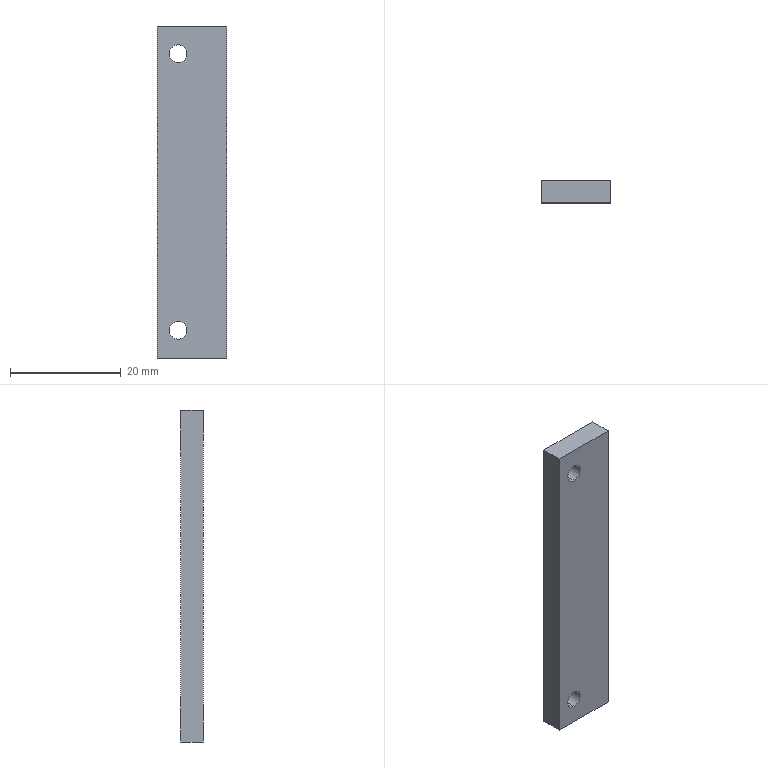Part | STEP file | PN_0027 | 1 solid | 14 faces | box 12.5 x 4 x 60 mm | volume 2901 mm3 | plane 6 | cone 4 | cylinder 4 | commonest cylinder face diameters 3.2 x4
STEP:
#1=CARTESIAN_POINT('',(0.,0.,0.));
#2=DIRECTION('',(0.,0.,1.));
#3=DIRECTION('',(1.,0.,0.));
#4=AXIS2_PLACEMENT_3D('',#1,#2,#3);
#5=CARTESIAN_POINT('',(-2.5,2.4,-23.4));
#6=VERTEX_POINT('',#5);
#7=CARTESIAN_POINT('',(-2.5,4.,-21.8));
#8=VERTEX_POINT('',#7);
#9=CARTESIAN_POINT('',(-2.5,4.,-21.8));
#10=DIRECTION('',(0.,0.7071,0.7071));
#11=VECTOR('',#10,1.);
#12=LINE('',#9,#11);
#13=CARTESIAN_POINT('',(-2.5,4.,-25.));
#14=DIRECTION('',(0.,1.,0.));
#15=DIRECTION('',(0.,0.,1.));
#16=AXIS2_PLACEMENT_3D('',#13,#14,#15);
#17=CONICAL_SURFACE('',#16,3.2,0.7854);
#18=CARTESIAN_POINT('',(6.283,0.));
#19=DIRECTION('',(0.,1.));
#20=VECTOR('',#19,1.);
#21=LINE('',#18,#20);
#22=(GEOMETRIC_REPRESENTATION_CONTEXT(2)PARAMETRIC_REPRESENTATION_CONTEXT()REPRESENTATION_CONTEXT('',''));
#23=DEFINITIONAL_REPRESENTATION('',(#21),#22);
#24=PCURVE('',#17,#23);
#25=CARTESIAN_POINT('',(-2.5,4.,-25.));
#26=DIRECTION('',(0.,1.,0.));
#27=DIRECTION('',(0.,0.,1.));
#28=AXIS2_PLACEMENT_3D('',#25,#26,#27);
#29=CONICAL_SURFACE('',#28,3.2,0.7854);
#30=CARTESIAN_POINT('',(0.,0.));
#31=DIRECTION('',(0.,1.));
#32=VECTOR('',#31,1.);
#33=LINE('',#30,#32);
#34=(GEOMETRIC_REPRESENTATION_CONTEXT(2)PARAMETRIC_REPRESENTATION_CONTEXT()REPRESENTATION_CONTEXT('',''));
#35=DEFINITIONAL_REPRESENTATION('',(#33),#34);
#36=PCURVE('',#29,#35);
#37=SURFACE_CURVE('',#12,(#24,#36),.PCURVE_S1.);
#38=EDGE_CURVE('',#6,#8,#37,.T.);
#39=ORIENTED_EDGE('',*,*,#38,.T.);
#40=CARTESIAN_POINT('',(-2.5,4.,-28.2));
#41=VERTEX_POINT('',#40);
#42=CARTESIAN_POINT('',(-2.5,4.,-25.));
#43=DIRECTION('',(0.,1.,0.));
#44=DIRECTION('',(0.,0.,1.));
#45=AXIS2_PLACEMENT_3D('',#42,#43,#44);
#46=CIRCLE('',#45,3.2);
#47=CARTESIAN_POINT('',(0.,0.));
#48=DIRECTION('',(1.,0.));
#49=VECTOR('',#48,1.);
#50=LINE('',#47,#49);
#51=(GEOMETRIC_REPRESENTATION_CONTEXT(2)PARAMETRIC_REPRESENTATION_CONTEXT()REPRESENTATION_CONTEXT('',''));
#52=DEFINITIONAL_REPRESENTATION('',(#50),#51);
#53=PCURVE('',#17,#52);
#54=CARTESIAN_POINT('',(0.,4.,0.));
#55=DIRECTION('',(0.,1.,0.));
#56=DIRECTION('',(0.,0.,1.));
#57=AXIS2_PLACEMENT_3D('',#54,#55,#56);
#58=PLANE('',#57);
#59=CARTESIAN_POINT('',(-25.,-2.5));
#60=DIRECTION('',(1.,0.));
#61=AXIS2_PLACEMENT_2D('',#59,#60);
#62=CIRCLE('',#61,3.2);
#63=(GEOMETRIC_REPRESENTATION_CONTEXT(2)PARAMETRIC_REPRESENTATION_CONTEXT()REPRESENTATION_CONTEXT('',''));
#64=DEFINITIONAL_REPRESENTATION('',(#62),#63);
#65=PCURVE('',#58,#64);
#66=SURFACE_CURVE('',#46,(#53,#65),.PCURVE_S1.);
#67=EDGE_CURVE('',#41,#8,#66,.T.);
#68=ORIENTED_EDGE('',*,*,#67,.F.);
#69=CARTESIAN_POINT('',(-2.5,2.4,-26.6));
#70=VERTEX_POINT('',#69);
#71=CARTESIAN_POINT('',(-2.5,4.,-28.2));
#72=DIRECTION('',(0.,0.7071,-0.7071));
#73=VECTOR('',#72,1.);
#74=LINE('',#71,#73);
#75=CARTESIAN_POINT('',(3.142,0.));
#76=DIRECTION('',(0.,1.));
#77=VECTOR('',#76,1.);
#78=LINE('',#75,#77);
#79=(GEOMETRIC_REPRESENTATION_CONTEXT(2)PARAMETRIC_REPRESENTATION_CONTEXT()REPRESENTATION_CONTEXT('',''));
#80=DEFINITIONAL_REPRESENTATION('',(#78),#79);
#81=PCURVE('',#17,#80);
#82=CARTESIAN_POINT('',(3.142,0.));
#83=DIRECTION('',(0.,1.));
#84=VECTOR('',#83,1.);
#85=LINE('',#82,#84);
#86=(GEOMETRIC_REPRESENTATION_CONTEXT(2)PARAMETRIC_REPRESENTATION_CONTEXT()REPRESENTATION_CONTEXT('',''));
#87=DEFINITIONAL_REPRESENTATION('',(#85),#86);
#88=PCURVE('',#29,#87);
#89=SURFACE_CURVE('',#74,(#81,#88),.PCURVE_S1.);
#90=EDGE_CURVE('',#70,#41,#89,.T.);
#91=ORIENTED_EDGE('',*,*,#90,.F.);
#92=CARTESIAN_POINT('',(-2.5,2.4,-25.));
#93=DIRECTION('',(0.,1.,0.));
#94=DIRECTION('',(0.,0.,1.));
#95=AXIS2_PLACEMENT_3D('',#92,#93,#94);
#96=CIRCLE('',#95,1.6);
#97=CARTESIAN_POINT('',(0.,-1.6));
#98=DIRECTION('',(1.,0.));
#99=VECTOR('',#98,1.);
#100=LINE('',#97,#99);
#101=(GEOMETRIC_REPRESENTATION_CONTEXT(2)PARAMETRIC_REPRESENTATION_CONTEXT()REPRESENTATION_CONTEXT('',''));
#102=DEFINITIONAL_REPRESENTATION('',(#100),#101);
#103=PCURVE('',#17,#102);
#104=CARTESIAN_POINT('',(-2.5,4.,-25.));
#105=DIRECTION('',(0.,1.,0.));
#106=DIRECTION('',(0.,0.,1.));
#107=AXIS2_PLACEMENT_3D('',#104,#105,#106);
#108=CYLINDRICAL_SURFACE('',#107,1.6);
#109=CARTESIAN_POINT('',(0.,-1.6));
#110=DIRECTION('',(1.,0.));
#111=VECTOR('',#110,1.);
#112=LINE('',#109,#111);
#113=(GEOMETRIC_REPRESENTATION_CONTEXT(2)PARAMETRIC_REPRESENTATION_CONTEXT()REPRESENTATION_CONTEXT('',''));
#114=DEFINITIONAL_REPRESENTATION('',(#112),#113);
#115=PCURVE('',#108,#114);
#116=SURFACE_CURVE('',#96,(#103,#115),.PCURVE_S1.);
#117=EDGE_CURVE('',#70,#6,#116,.T.);
#118=ORIENTED_EDGE('',*,*,#117,.T.);
#119=EDGE_LOOP('',(#39,#68,#91,#118));
#120=FACE_BOUND('',#119,.F.);
#121=ADVANCED_FACE('',(#120),#17,.F.);
#122=CARTESIAN_POINT('',(-2.5,0.,-23.4));
#123=VERTEX_POINT('',#122);
#124=CARTESIAN_POINT('',(-2.5,4.,-23.4));
#125=DIRECTION('',(0.,1.,0.));
#126=VECTOR('',#125,1.);
#127=LINE('',#124,#126);
#128=CARTESIAN_POINT('',(6.283,0.));
#129=DIRECTION('',(0.,1.));
#130=VECTOR('',#129,1.);
#131=LINE('',#128,#130);
#132=(GEOMETRIC_REPRESENTATION_CONTEXT(2)PARAMETRIC_REPRESENTATION_CONTEXT()REPRESENTATION_CONTEXT('',''));
#133=DEFINITIONAL_REPRESENTATION('',(#131),#132);
#134=PCURVE('',#108,#133);
#135=CARTESIAN_POINT('',(-2.5,4.,-25.));
#136=DIRECTION('',(0.,1.,0.));
#137=DIRECTION('',(0.,0.,1.));
#138=AXIS2_PLACEMENT_3D('',#135,#136,#137);
#139=CYLINDRICAL_SURFACE('',#138,1.6);
#140=CARTESIAN_POINT('',(0.,0.));
#141=DIRECTION('',(0.,1.));
#142=VECTOR('',#141,1.);
#143=LINE('',#140,#142);
#144=(GEOMETRIC_REPRESENTATION_CONTEXT(2)PARAMETRIC_REPRESENTATION_CONTEXT()REPRESENTATION_CONTEXT('',''));
#145=DEFINITIONAL_REPRESENTATION('',(#143),#144);
#146=PCURVE('',#139,#145);
#147=SURFACE_CURVE('',#127,(#134,#146),.PCURVE_S1.);
#148=EDGE_CURVE('',#123,#6,#147,.T.);
#149=ORIENTED_EDGE('',*,*,#148,.T.);
#150=ORIENTED_EDGE('',*,*,#117,.F.);
#151=CARTESIAN_POINT('',(-2.5,0.,-26.6));
#152=VERTEX_POINT('',#151);
#153=CARTESIAN_POINT('',(-2.5,4.,-26.6));
#154=DIRECTION('',(0.,1.,0.));
#155=VECTOR('',#154,1.);
#156=LINE('',#153,#155);
#157=CARTESIAN_POINT('',(3.142,0.));
#158=DIRECTION('',(0.,1.));
#159=VECTOR('',#158,1.);
#160=LINE('',#157,#159);
#161=(GEOMETRIC_REPRESENTATION_CONTEXT(2)PARAMETRIC_REPRESENTATION_CONTEXT()REPRESENTATION_CONTEXT('',''));
#162=DEFINITIONAL_REPRESENTATION('',(#160),#161);
#163=PCURVE('',#108,#162);
#164=CARTESIAN_POINT('',(3.142,0.));
#165=DIRECTION('',(0.,1.));
#166=VECTOR('',#165,1.);
#167=LINE('',#164,#166);
#168=(GEOMETRIC_REPRESENTATION_CONTEXT(2)PARAMETRIC_REPRESENTATION_CONTEXT()REPRESENTATION_CONTEXT('',''));
#169=DEFINITIONAL_REPRESENTATION('',(#167),#168);
#170=PCURVE('',#139,#169);
#171=SURFACE_CURVE('',#156,(#163,#170),.PCURVE_S1.);
#172=EDGE_CURVE('',#152,#70,#171,.T.);
#173=ORIENTED_EDGE('',*,*,#172,.F.);
#174=CARTESIAN_POINT('',(-2.5,0.,-25.));
#175=DIRECTION('',(0.,1.,0.));
#176=DIRECTION('',(0.,0.,1.));
#177=AXIS2_PLACEMENT_3D('',#174,#175,#176);
#178=CIRCLE('',#177,1.6);
#179=CARTESIAN_POINT('',(0.,-4.));
#180=DIRECTION('',(1.,0.));
#181=VECTOR('',#180,1.);
#182=LINE('',#179,#181);
#183=(GEOMETRIC_REPRESENTATION_CONTEXT(2)PARAMETRIC_REPRESENTATION_CONTEXT()REPRESENTATION_CONTEXT('',''));
#184=DEFINITIONAL_REPRESENTATION('',(#182),#183);
#185=PCURVE('',#108,#184);
#186=CARTESIAN_POINT('',(0.,0.,0.));
#187=DIRECTION('',(0.,1.,0.));
#188=DIRECTION('',(0.,0.,1.));
#189=AXIS2_PLACEMENT_3D('',#186,#187,#188);
#190=PLANE('',#189);
#191=CARTESIAN_POINT('',(-25.,-2.5));
#192=DIRECTION('',(1.,0.));
#193=AXIS2_PLACEMENT_2D('',#191,#192);
#194=CIRCLE('',#193,1.6);
#195=(GEOMETRIC_REPRESENTATION_CONTEXT(2)PARAMETRIC_REPRESENTATION_CONTEXT()REPRESENTATION_CONTEXT('',''));
#196=DEFINITIONAL_REPRESENTATION('',(#194),#195);
#197=PCURVE('',#190,#196);
#198=SURFACE_CURVE('',#178,(#185,#197),.PCURVE_S1.);
#199=EDGE_CURVE('',#152,#123,#198,.T.);
#200=ORIENTED_EDGE('',*,*,#199,.T.);
#201=EDGE_LOOP('',(#149,#150,#173,#200));
#202=FACE_BOUND('',#201,.F.);
#203=ADVANCED_FACE('',(#202),#108,.F.);
#204=CARTESIAN_POINT('',(-2.5,2.4,26.6));
#205=VERTEX_POINT('',#204);
#206=CARTESIAN_POINT('',(-2.5,4.,28.2));
#207=VERTEX_POINT('',#206);
#208=CARTESIAN_POINT('',(-2.5,4.,28.2));
#209=DIRECTION('',(0.,0.7071,0.7071));
#210=VECTOR('',#209,1.);
#211=LINE('',#208,#210);
#212=CARTESIAN_POINT('',(-2.5,4.,25.));
#213=DIRECTION('',(0.,1.,0.));
#214=DIRECTION('',(0.,0.,1.));
#215=AXIS2_PLACEMENT_3D('',#212,#213,#214);
#216=CONICAL_SURFACE('',#215,3.2,0.7854);
#217=CARTESIAN_POINT('',(6.283,0.));
#218=DIRECTION('',(0.,1.));
#219=VECTOR('',#218,1.);
#220=LINE('',#217,#219);
#221=(GEOMETRIC_REPRESENTATION_CONTEXT(2)PARAMETRIC_REPRESENTATION_CONTEXT()REPRESENTATION_CONTEXT('',''));
#222=DEFINITIONAL_REPRESENTATION('',(#220),#221);
#223=PCURVE('',#216,#222);
#224=CARTESIAN_POINT('',(-2.5,4.,25.));
#225=DIRECTION('',(0.,1.,0.));
#226=DIRECTION('',(0.,0.,1.));
#227=AXIS2_PLACEMENT_3D('',#224,#225,#226);
#228=CONICAL_SURFACE('',#227,3.2,0.7854);
#229=CARTESIAN_POINT('',(0.,0.));
#230=DIRECTION('',(0.,1.));
#231=VECTOR('',#230,1.);
#232=LINE('',#229,#231);
#233=(GEOMETRIC_REPRESENTATION_CONTEXT(2)PARAMETRIC_REPRESENTATION_CONTEXT()REPRESENTATION_CONTEXT('',''));
#234=DEFINITIONAL_REPRESENTATION('',(#232),#233);
#235=PCURVE('',#228,#234);
#236=SURFACE_CURVE('',#211,(#223,#235),.PCURVE_S1.);
#237=EDGE_CURVE('',#205,#207,#236,.T.);
#238=ORIENTED_EDGE('',*,*,#237,.T.);
#239=CARTESIAN_POINT('',(-2.5,4.,21.8));
#240=VERTEX_POINT('',#239);
#241=CARTESIAN_POINT('',(-2.5,4.,25.));
#242=DIRECTION('',(0.,1.,0.));
#243=DIRECTION('',(0.,0.,1.));
#244=AXIS2_PLACEMENT_3D('',#241,#242,#243);
#245=CIRCLE('',#244,3.2);
#246=CARTESIAN_POINT('',(0.,0.));
#247=DIRECTION('',(1.,0.));
#248=VECTOR('',#247,1.);
#249=LINE('',#246,#248);
#250=(GEOMETRIC_REPRESENTATION_CONTEXT(2)PARAMETRIC_REPRESENTATION_CONTEXT()REPRESENTATION_CONTEXT('',''));
#251=DEFINITIONAL_REPRESENTATION('',(#249),#250);
#252=PCURVE('',#216,#251);
#253=CARTESIAN_POINT('',(25.,-2.5));
#254=DIRECTION('',(1.,0.));
#255=AXIS2_PLACEMENT_2D('',#253,#254);
#256=CIRCLE('',#255,3.2);
#257=(GEOMETRIC_REPRESENTATION_CONTEXT(2)PARAMETRIC_REPRESENTATION_CONTEXT()REPRESENTATION_CONTEXT('',''));
#258=DEFINITIONAL_REPRESENTATION('',(#256),#257);
#259=PCURVE('',#58,#258);
#260=SURFACE_CURVE('',#245,(#252,#259),.PCURVE_S1.);
#261=EDGE_CURVE('',#240,#207,#260,.T.);
#262=ORIENTED_EDGE('',*,*,#261,.F.);
#263=CARTESIAN_POINT('',(-2.5,2.4,23.4));
#264=VERTEX_POINT('',#263);
#265=CARTESIAN_POINT('',(-2.5,4.,21.8));
#266=DIRECTION('',(0.,0.7071,-0.7071));
#267=VECTOR('',#266,1.);
#268=LINE('',#265,#267);
#269=CARTESIAN_POINT('',(3.142,0.));
#270=DIRECTION('',(0.,1.));
#271=VECTOR('',#270,1.);
#272=LINE('',#269,#271);
#273=(GEOMETRIC_REPRESENTATION_CONTEXT(2)PARAMETRIC_REPRESENTATION_CONTEXT()REPRESENTATION_CONTEXT('',''));
#274=DEFINITIONAL_REPRESENTATION('',(#272),#273);
#275=PCURVE('',#216,#274);
#276=CARTESIAN_POINT('',(3.142,0.));
#277=DIRECTION('',(0.,1.));
#278=VECTOR('',#277,1.);
#279=LINE('',#276,#278);
#280=(GEOMETRIC_REPRESENTATION_CONTEXT(2)PARAMETRIC_REPRESENTATION_CONTEXT()REPRESENTATION_CONTEXT('',''));
#281=DEFINITIONAL_REPRESENTATION('',(#279),#280);
#282=PCURVE('',#228,#281);
#283=SURFACE_CURVE('',#268,(#275,#282),.PCURVE_S1.);
#284=EDGE_CURVE('',#264,#240,#283,.T.);
#285=ORIENTED_EDGE('',*,*,#284,.F.);
#286=CARTESIAN_POINT('',(-2.5,2.4,25.));
#287=DIRECTION('',(0.,1.,0.));
#288=DIRECTION('',(0.,0.,1.));
#289=AXIS2_PLACEMENT_3D('',#286,#287,#288);
#290=CIRCLE('',#289,1.6);
#291=CARTESIAN_POINT('',(0.,-1.6));
#292=DIRECTION('',(1.,0.));
#293=VECTOR('',#292,1.);
#294=LINE('',#291,#293);
#295=(GEOMETRIC_REPRESENTATION_CONTEXT(2)PARAMETRIC_REPRESENTATION_CONTEXT()REPRESENTATION_CONTEXT('',''));
#296=DEFINITIONAL_REPRESENTATION('',(#294),#295);
#297=PCURVE('',#216,#296);
#298=CARTESIAN_POINT('',(-2.5,4.,25.));
#299=DIRECTION('',(0.,1.,0.));
#300=DIRECTION('',(0.,0.,1.));
#301=AXIS2_PLACEMENT_3D('',#298,#299,#300);
#302=CYLINDRICAL_SURFACE('',#301,1.6);
#303=CARTESIAN_POINT('',(0.,-1.6));
#304=DIRECTION('',(1.,0.));
#305=VECTOR('',#304,1.);
#306=LINE('',#303,#305);
#307=(GEOMETRIC_REPRESENTATION_CONTEXT(2)PARAMETRIC_REPRESENTATION_CONTEXT()REPRESENTATION_CONTEXT('',''));
#308=DEFINITIONAL_REPRESENTATION('',(#306),#307);
#309=PCURVE('',#302,#308);
#310=SURFACE_CURVE('',#290,(#297,#309),.PCURVE_S1.);
#311=EDGE_CURVE('',#264,#205,#310,.T.);
#312=ORIENTED_EDGE('',*,*,#311,.T.);
#313=EDGE_LOOP('',(#238,#262,#285,#312));
#314=FACE_BOUND('',#313,.F.);
#315=ADVANCED_FACE('',(#314),#216,.F.);
#316=CARTESIAN_POINT('',(-2.5,0.,26.6));
#317=VERTEX_POINT('',#316);
#318=CARTESIAN_POINT('',(-2.5,4.,26.6));
#319=DIRECTION('',(0.,1.,0.));
#320=VECTOR('',#319,1.);
#321=LINE('',#318,#320);
#322=CARTESIAN_POINT('',(6.283,0.));
#323=DIRECTION('',(0.,1.));
#324=VECTOR('',#323,1.);
#325=LINE('',#322,#324);
#326=(GEOMETRIC_REPRESENTATION_CONTEXT(2)PARAMETRIC_REPRESENTATION_CONTEXT()REPRESENTATION_CONTEXT('',''));
#327=DEFINITIONAL_REPRESENTATION('',(#325),#326);
#328=PCURVE('',#302,#327);
#329=CARTESIAN_POINT('',(-2.5,4.,25.));
#330=DIRECTION('',(0.,1.,0.));
#331=DIRECTION('',(0.,0.,1.));
#332=AXIS2_PLACEMENT_3D('',#329,#330,#331);
#333=CYLINDRICAL_SURFACE('',#332,1.6);
#334=CARTESIAN_POINT('',(0.,0.));
#335=DIRECTION('',(0.,1.));
#336=VECTOR('',#335,1.);
#337=LINE('',#334,#336);
#338=(GEOMETRIC_REPRESENTATION_CONTEXT(2)PARAMETRIC_REPRESENTATION_CONTEXT()REPRESENTATION_CONTEXT('',''));
#339=DEFINITIONAL_REPRESENTATION('',(#337),#338);
#340=PCURVE('',#333,#339);
#341=SURFACE_CURVE('',#321,(#328,#340),.PCURVE_S1.);
#342=EDGE_CURVE('',#317,#205,#341,.T.);
#343=ORIENTED_EDGE('',*,*,#342,.T.);
#344=ORIENTED_EDGE('',*,*,#311,.F.);
#345=CARTESIAN_POINT('',(-2.5,0.,23.4));
#346=VERTEX_POINT('',#345);
#347=CARTESIAN_POINT('',(-2.5,4.,23.4));
#348=DIRECTION('',(0.,1.,0.));
#349=VECTOR('',#348,1.);
#350=LINE('',#347,#349);
#351=CARTESIAN_POINT('',(3.142,0.));
#352=DIRECTION('',(0.,1.));
#353=VECTOR('',#352,1.);
#354=LINE('',#351,#353);
#355=(GEOMETRIC_REPRESENTATION_CONTEXT(2)PARAMETRIC_REPRESENTATION_CONTEXT()REPRESENTATION_CONTEXT('',''));
#356=DEFINITIONAL_REPRESENTATION('',(#354),#355);
#357=PCURVE('',#302,#356);
#358=CARTESIAN_POINT('',(3.142,0.));
#359=DIRECTION('',(0.,1.));
#360=VECTOR('',#359,1.);
#361=LINE('',#358,#360);
#362=(GEOMETRIC_REPRESENTATION_CONTEXT(2)PARAMETRIC_REPRESENTATION_CONTEXT()REPRESENTATION_CONTEXT('',''));
#363=DEFINITIONAL_REPRESENTATION('',(#361),#362);
#364=PCURVE('',#333,#363);
#365=SURFACE_CURVE('',#350,(#357,#364),.PCURVE_S1.);
#366=EDGE_CURVE('',#346,#264,#365,.T.);
#367=ORIENTED_EDGE('',*,*,#366,.F.);
#368=CARTESIAN_POINT('',(-2.5,0.,25.));
#369=DIRECTION('',(0.,1.,0.));
#370=DIRECTION('',(0.,0.,1.));
#371=AXIS2_PLACEMENT_3D('',#368,#369,#370);
#372=CIRCLE('',#371,1.6);
#373=CARTESIAN_POINT('',(0.,-4.));
#374=DIRECTION('',(1.,0.));
#375=VECTOR('',#374,1.);
#376=LINE('',#373,#375);
#377=(GEOMETRIC_REPRESENTATION_CONTEXT(2)PARAMETRIC_REPRESENTATION_CONTEXT()REPRESENTATION_CONTEXT('',''));
#378=DEFINITIONAL_REPRESENTATION('',(#376),#377);
#379=PCURVE('',#302,#378);
#380=CARTESIAN_POINT('',(25.,-2.5));
#381=DIRECTION('',(1.,0.));
#382=AXIS2_PLACEMENT_2D('',#380,#381);
#383=CIRCLE('',#382,1.6);
#384=(GEOMETRIC_REPRESENTATION_CONTEXT(2)PARAMETRIC_REPRESENTATION_CONTEXT()REPRESENTATION_CONTEXT('',''));
#385=DEFINITIONAL_REPRESENTATION('',(#383),#384);
#386=PCURVE('',#190,#385);
#387=SURFACE_CURVE('',#372,(#379,#386),.PCURVE_S1.);
#388=EDGE_CURVE('',#346,#317,#387,.T.);
#389=ORIENTED_EDGE('',*,*,#388,.T.);
#390=EDGE_LOOP('',(#343,#344,#367,#389));
#391=FACE_BOUND('',#390,.F.);
#392=ADVANCED_FACE('',(#391),#302,.F.);
#393=CARTESIAN_POINT('',(6.25,0.,30.));
#394=VERTEX_POINT('',#393);
#395=CARTESIAN_POINT('',(6.25,0.,-30.));
#396=VERTEX_POINT('',#395);
#397=CARTESIAN_POINT('',(6.25,0.,-30.));
#398=DIRECTION('',(0.,0.,-1.));
#399=VECTOR('',#398,1.);
#400=LINE('',#397,#399);
#401=CARTESIAN_POINT('',(6.25,4.,-30.));
#402=DIRECTION('',(-1.,0.,0.));
#403=DIRECTION('',(0.,0.,1.));
#404=AXIS2_PLACEMENT_3D('',#401,#402,#403);
#405=PLANE('',#404);
#406=CARTESIAN_POINT('',(0.,-4.));
#407=DIRECTION('',(-1.,0.));
#408=VECTOR('',#407,1.);
#409=LINE('',#406,#408);
#410=(GEOMETRIC_REPRESENTATION_CONTEXT(2)PARAMETRIC_REPRESENTATION_CONTEXT()REPRESENTATION_CONTEXT('',''));
#411=DEFINITIONAL_REPRESENTATION('',(#409),#410);
#412=PCURVE('',#405,#411);
#413=CARTESIAN_POINT('',(-30.,6.25));
#414=DIRECTION('',(-1.,0.));
#415=VECTOR('',#414,1.);
#416=LINE('',#413,#415);
#417=(GEOMETRIC_REPRESENTATION_CONTEXT(2)PARAMETRIC_REPRESENTATION_CONTEXT()REPRESENTATION_CONTEXT('',''));
#418=DEFINITIONAL_REPRESENTATION('',(#416),#417);
#419=PCURVE('',#190,#418);
#420=SURFACE_CURVE('',#400,(#412,#419),.PCURVE_S1.);
#421=EDGE_CURVE('',#394,#396,#420,.T.);
#422=ORIENTED_EDGE('',*,*,#421,.T.);
#423=CARTESIAN_POINT('',(6.25,4.,-30.));
#424=VERTEX_POINT('',#423);
#425=CARTESIAN_POINT('',(6.25,4.,-30.));
#426=DIRECTION('',(0.,-1.,0.));
#427=VECTOR('',#426,1.);
#428=LINE('',#425,#427);
#429=CARTESIAN_POINT('',(0.,0.));
#430=DIRECTION('',(0.,-1.));
#431=VECTOR('',#430,1.);
#432=LINE('',#429,#431);
#433=(GEOMETRIC_REPRESENTATION_CONTEXT(2)PARAMETRIC_REPRESENTATION_CONTEXT()REPRESENTATION_CONTEXT('',''));
#434=DEFINITIONAL_REPRESENTATION('',(#432),#433);
#435=PCURVE('',#405,#434);
#436=CARTESIAN_POINT('',(-6.25,4.,-30.));
#437=DIRECTION('',(0.,0.,1.));
#438=DIRECTION('',(1.,0.,0.));
#439=AXIS2_PLACEMENT_3D('',#436,#437,#438);
#440=PLANE('',#439);
#441=CARTESIAN_POINT('',(12.5,0.));
#442=DIRECTION('',(0.,-1.));
#443=VECTOR('',#442,1.);
#444=LINE('',#441,#443);
#445=(GEOMETRIC_REPRESENTATION_CONTEXT(2)PARAMETRIC_REPRESENTATION_CONTEXT()REPRESENTATION_CONTEXT('',''));
#446=DEFINITIONAL_REPRESENTATION('',(#444),#445);
#447=PCURVE('',#440,#446);
#448=SURFACE_CURVE('',#428,(#435,#447),.PCURVE_S1.);
#449=EDGE_CURVE('',#424,#396,#448,.T.);
#450=ORIENTED_EDGE('',*,*,#449,.F.);
#451=CARTESIAN_POINT('',(6.25,4.,30.));
#452=VERTEX_POINT('',#451);
#453=CARTESIAN_POINT('',(6.25,4.,-30.));
#454=DIRECTION('',(0.,0.,-1.));
#455=VECTOR('',#454,1.);
#456=LINE('',#453,#455);
#457=CARTESIAN_POINT('',(0.,0.));
#458=DIRECTION('',(-1.,0.));
#459=VECTOR('',#458,1.);
#460=LINE('',#457,#459);
#461=(GEOMETRIC_REPRESENTATION_CONTEXT(2)PARAMETRIC_REPRESENTATION_CONTEXT()REPRESENTATION_CONTEXT('',''));
#462=DEFINITIONAL_REPRESENTATION('',(#460),#461);
#463=PCURVE('',#405,#462);
#464=CARTESIAN_POINT('',(-30.,6.25));
#465=DIRECTION('',(-1.,0.));
#466=VECTOR('',#465,1.);
#467=LINE('',#464,#466);
#468=(GEOMETRIC_REPRESENTATION_CONTEXT(2)PARAMETRIC_REPRESENTATION_CONTEXT()REPRESENTATION_CONTEXT('',''));
#469=DEFINITIONAL_REPRESENTATION('',(#467),#468);
#470=PCURVE('',#58,#469);
#471=SURFACE_CURVE('',#456,(#463,#470),.PCURVE_S1.);
#472=EDGE_CURVE('',#452,#424,#471,.T.);
#473=ORIENTED_EDGE('',*,*,#472,.F.);
#474=CARTESIAN_POINT('',(6.25,4.,30.));
#475=DIRECTION('',(0.,-1.,0.));
#476=VECTOR('',#475,1.);
#477=LINE('',#474,#476);
#478=CARTESIAN_POINT('',(60.,0.));
#479=DIRECTION('',(0.,-1.));
#480=VECTOR('',#479,1.);
#481=LINE('',#478,#480);
#482=(GEOMETRIC_REPRESENTATION_CONTEXT(2)PARAMETRIC_REPRESENTATION_CONTEXT()REPRESENTATION_CONTEXT('',''));
#483=DEFINITIONAL_REPRESENTATION('',(#481),#482);
#484=PCURVE('',#405,#483);
#485=CARTESIAN_POINT('',(-6.25,4.,30.));
#486=DIRECTION('',(0.,0.,-1.));
#487=DIRECTION('',(-1.,0.,0.));
#488=AXIS2_PLACEMENT_3D('',#485,#486,#487);
#489=PLANE('',#488);
#490=CARTESIAN_POINT('',(-12.5,0.));
#491=DIRECTION('',(0.,-1.));
#492=VECTOR('',#491,1.);
#493=LINE('',#490,#492);
#494=(GEOMETRIC_REPRESENTATION_CONTEXT(2)PARAMETRIC_REPRESENTATION_CONTEXT()REPRESENTATION_CONTEXT('',''));
#495=DEFINITIONAL_REPRESENTATION('',(#493),#494);
#496=PCURVE('',#489,#495);
#497=SURFACE_CURVE('',#477,(#484,#496),.PCURVE_S1.);
#498=EDGE_CURVE('',#452,#394,#497,.T.);
#499=ORIENTED_EDGE('',*,*,#498,.T.);
#500=EDGE_LOOP('',(#422,#450,#473,#499));
#501=FACE_BOUND('',#500,.T.);
#502=ADVANCED_FACE('',(#501),#405,.F.);
#503=CARTESIAN_POINT('',(-6.25,0.,-30.));
#504=VERTEX_POINT('',#503);
#505=CARTESIAN_POINT('',(-6.25,0.,-30.));
#506=DIRECTION('',(-1.,0.,0.));
#507=VECTOR('',#506,1.);
#508=LINE('',#505,#507);
#509=CARTESIAN_POINT('',(0.,-4.));
#510=DIRECTION('',(-1.,0.));
#511=VECTOR('',#510,1.);
#512=LINE('',#509,#511);
#513=(GEOMETRIC_REPRESENTATION_CONTEXT(2)PARAMETRIC_REPRESENTATION_CONTEXT()REPRESENTATION_CONTEXT('',''));
#514=DEFINITIONAL_REPRESENTATION('',(#512),#513);
#515=PCURVE('',#440,#514);
#516=CARTESIAN_POINT('',(-30.,-6.25));
#517=DIRECTION('',(0.,-1.));
#518=VECTOR('',#517,1.);
#519=LINE('',#516,#518);
#520=(GEOMETRIC_REPRESENTATION_CONTEXT(2)PARAMETRIC_REPRESENTATION_CONTEXT()REPRESENTATION_CONTEXT('',''));
#521=DEFINITIONAL_REPRESENTATION('',(#519),#520);
#522=PCURVE('',#190,#521);
#523=SURFACE_CURVE('',#508,(#515,#522),.PCURVE_S1.);
#524=EDGE_CURVE('',#396,#504,#523,.T.);
#525=ORIENTED_EDGE('',*,*,#524,.T.);
#526=CARTESIAN_POINT('',(-6.25,4.,-30.));
#527=VERTEX_POINT('',#526);
#528=CARTESIAN_POINT('',(-6.25,4.,-30.));
#529=DIRECTION('',(0.,-1.,0.));
#530=VECTOR('',#529,1.);
#531=LINE('',#528,#530);
#532=CARTESIAN_POINT('',(0.,0.));
#533=DIRECTION('',(0.,-1.));
#534=VECTOR('',#533,1.);
#535=LINE('',#532,#534);
#536=(GEOMETRIC_REPRESENTATION_CONTEXT(2)PARAMETRIC_REPRESENTATION_CONTEXT()REPRESENTATION_CONTEXT('',''));
#537=DEFINITIONAL_REPRESENTATION('',(#535),#536);
#538=PCURVE('',#440,#537);
#539=CARTESIAN_POINT('',(-6.25,4.,-30.));
#540=DIRECTION('',(1.,0.,0.));
#541=DIRECTION('',(0.,0.,-1.));
#542=AXIS2_PLACEMENT_3D('',#539,#540,#541);
#543=PLANE('',#542);
#544=CARTESIAN_POINT('',(0.,0.));
#545=DIRECTION('',(0.,-1.));
#546=VECTOR('',#545,1.);
#547=LINE('',#544,#546);
#548=(GEOMETRIC_REPRESENTATION_CONTEXT(2)PARAMETRIC_REPRESENTATION_CONTEXT()REPRESENTATION_CONTEXT('',''));
#549=DEFINITIONAL_REPRESENTATION('',(#547),#548);
#550=PCURVE('',#543,#549);
#551=SURFACE_CURVE('',#531,(#538,#550),.PCURVE_S1.);
#552=EDGE_CURVE('',#527,#504,#551,.T.);
#553=ORIENTED_EDGE('',*,*,#552,.F.);
#554=CARTESIAN_POINT('',(-6.25,4.,-30.));
#555=DIRECTION('',(-1.,0.,0.));
#556=VECTOR('',#555,1.);
#557=LINE('',#554,#556);
#558=CARTESIAN_POINT('',(0.,0.));
#559=DIRECTION('',(-1.,0.));
#560=VECTOR('',#559,1.);
#561=LINE('',#558,#560);
#562=(GEOMETRIC_REPRESENTATION_CONTEXT(2)PARAMETRIC_REPRESENTATION_CONTEXT()REPRESENTATION_CONTEXT('',''));
#563=DEFINITIONAL_REPRESENTATION('',(#561),#562);
#564=PCURVE('',#440,#563);
#565=CARTESIAN_POINT('',(-30.,-6.25));
#566=DIRECTION('',(0.,-1.));
#567=VECTOR('',#566,1.);
#568=LINE('',#565,#567);
#569=(GEOMETRIC_REPRESENTATION_CONTEXT(2)PARAMETRIC_REPRESENTATION_CONTEXT()REPRESENTATION_CONTEXT('',''));
#570=DEFINITIONAL_REPRESENTATION('',(#568),#569);
#571=PCURVE('',#58,#570);
#572=SURFACE_CURVE('',#557,(#564,#571),.PCURVE_S1.);
#573=EDGE_CURVE('',#424,#527,#572,.T.);
#574=ORIENTED_EDGE('',*,*,#573,.F.);
#575=ORIENTED_EDGE('',*,*,#449,.T.);
#576=EDGE_LOOP('',(#525,#553,#574,#575));
#577=FACE_BOUND('',#576,.T.);
#578=ADVANCED_FACE('',(#577),#440,.F.);
#579=CARTESIAN_POINT('',(-6.25,0.,30.));
#580=VERTEX_POINT('',#579);
#581=CARTESIAN_POINT('',(-6.25,0.,-30.));
#582=DIRECTION('',(0.,0.,1.));
#583=VECTOR('',#582,1.);
#584=LINE('',#581,#583);
#585=CARTESIAN_POINT('',(0.,-4.));
#586=DIRECTION('',(-1.,0.));
#587=VECTOR('',#586,1.);
#588=LINE('',#585,#587);
#589=(GEOMETRIC_REPRESENTATION_CONTEXT(2)PARAMETRIC_REPRESENTATION_CONTEXT()REPRESENTATION_CONTEXT('',''));
#590=DEFINITIONAL_REPRESENTATION('',(#588),#589);
#591=PCURVE('',#543,#590);
#592=CARTESIAN_POINT('',(-30.,-6.25));
#593=DIRECTION('',(1.,0.));
#594=VECTOR('',#593,1.);
#595=LINE('',#592,#594);
#596=(GEOMETRIC_REPRESENTATION_CONTEXT(2)PARAMETRIC_REPRESENTATION_CONTEXT()REPRESENTATION_CONTEXT('',''));
#597=DEFINITIONAL_REPRESENTATION('',(#595),#596);
#598=PCURVE('',#190,#597);
#599=SURFACE_CURVE('',#584,(#591,#598),.PCURVE_S1.);
#600=EDGE_CURVE('',#504,#580,#599,.T.);
#601=ORIENTED_EDGE('',*,*,#600,.T.);
#602=CARTESIAN_POINT('',(-6.25,4.,30.));
#603=VERTEX_POINT('',#602);
#604=CARTESIAN_POINT('',(-6.25,4.,30.));
#605=DIRECTION('',(0.,-1.,0.));
#606=VECTOR('',#605,1.);
#607=LINE('',#604,#606);
#608=CARTESIAN_POINT('',(-60.,0.));
#609=DIRECTION('',(0.,-1.));
#610=VECTOR('',#609,1.);
#611=LINE('',#608,#610);
#612=(GEOMETRIC_REPRESENTATION_CONTEXT(2)PARAMETRIC_REPRESENTATION_CONTEXT()REPRESENTATION_CONTEXT('',''));
#613=DEFINITIONAL_REPRESENTATION('',(#611),#612);
#614=PCURVE('',#543,#613);
#615=CARTESIAN_POINT('',(0.,0.));
#616=DIRECTION('',(0.,-1.));
#617=VECTOR('',#616,1.);
#618=LINE('',#615,#617);
#619=(GEOMETRIC_REPRESENTATION_CONTEXT(2)PARAMETRIC_REPRESENTATION_CONTEXT()REPRESENTATION_CONTEXT('',''));
#620=DEFINITIONAL_REPRESENTATION('',(#618),#619);
#621=PCURVE('',#489,#620);
#622=SURFACE_CURVE('',#607,(#614,#621),.PCURVE_S1.);
#623=EDGE_CURVE('',#603,#580,#622,.T.);
#624=ORIENTED_EDGE('',*,*,#623,.F.);
#625=CARTESIAN_POINT('',(-6.25,4.,-30.));
#626=DIRECTION('',(0.,0.,1.));
#627=VECTOR('',#626,1.);
#628=LINE('',#625,#627);
#629=CARTESIAN_POINT('',(0.,0.));
#630=DIRECTION('',(-1.,0.));
#631=VECTOR('',#630,1.);
#632=LINE('',#629,#631);
#633=(GEOMETRIC_REPRESENTATION_CONTEXT(2)PARAMETRIC_REPRESENTATION_CONTEXT()REPRESENTATION_CONTEXT('',''));
#634=DEFINITIONAL_REPRESENTATION('',(#632),#633);
#635=PCURVE('',#543,#634);
#636=CARTESIAN_POINT('',(-30.,-6.25));
#637=DIRECTION('',(1.,0.));
#638=VECTOR('',#637,1.);
#639=LINE('',#636,#638);
#640=(GEOMETRIC_REPRESENTATION_CONTEXT(2)PARAMETRIC_REPRESENTATION_CONTEXT()REPRESENTATION_CONTEXT('',''));
#641=DEFINITIONAL_REPRESENTATION('',(#639),#640);
#642=PCURVE('',#58,#641);
#643=SURFACE_CURVE('',#628,(#635,#642),.PCURVE_S1.);
#644=EDGE_CURVE('',#527,#603,#643,.T.);
#645=ORIENTED_EDGE('',*,*,#644,.F.);
#646=ORIENTED_EDGE('',*,*,#552,.T.);
#647=EDGE_LOOP('',(#601,#624,#645,#646));
#648=FACE_BOUND('',#647,.T.);
#649=ADVANCED_FACE('',(#648),#543,.F.);
#650=CARTESIAN_POINT('',(-6.25,0.,30.));
#651=DIRECTION('',(1.,0.,0.));
#652=VECTOR('',#651,1.);
#653=LINE('',#650,#652);
#654=CARTESIAN_POINT('',(0.,-4.));
#655=DIRECTION('',(-1.,0.));
#656=VECTOR('',#655,1.);
#657=LINE('',#654,#656);
#658=(GEOMETRIC_REPRESENTATION_CONTEXT(2)PARAMETRIC_REPRESENTATION_CONTEXT()REPRESENTATION_CONTEXT('',''));
#659=DEFINITIONAL_REPRESENTATION('',(#657),#658);
#660=PCURVE('',#489,#659);
#661=CARTESIAN_POINT('',(30.,-6.25));
#662=DIRECTION('',(0.,1.));
#663=VECTOR('',#662,1.);
#664=LINE('',#661,#663);
#665=(GEOMETRIC_REPRESENTATION_CONTEXT(2)PARAMETRIC_REPRESENTATION_CONTEXT()REPRESENTATION_CONTEXT('',''));
#666=DEFINITIONAL_REPRESENTATION('',(#664),#665);
#667=PCURVE('',#190,#666);
#668=SURFACE_CURVE('',#653,(#660,#667),.PCURVE_S1.);
#669=EDGE_CURVE('',#580,#394,#668,.T.);
#670=ORIENTED_EDGE('',*,*,#669,.T.);
#671=ORIENTED_EDGE('',*,*,#498,.F.);
#672=CARTESIAN_POINT('',(-6.25,4.,30.));
#673=DIRECTION('',(1.,0.,0.));
#674=VECTOR('',#673,1.);
#675=LINE('',#672,#674);
#676=CARTESIAN_POINT('',(0.,0.));
#677=DIRECTION('',(-1.,0.));
#678=VECTOR('',#677,1.);
#679=LINE('',#676,#678);
#680=(GEOMETRIC_REPRESENTATION_CONTEXT(2)PARAMETRIC_REPRESENTATION_CONTEXT()REPRESENTATION_CONTEXT('',''));
#681=DEFINITIONAL_REPRESENTATION('',(#679),#680);
#682=PCURVE('',#489,#681);
#683=CARTESIAN_POINT('',(30.,-6.25));
#684=DIRECTION('',(0.,1.));
#685=VECTOR('',#684,1.);
#686=LINE('',#683,#685);
#687=(GEOMETRIC_REPRESENTATION_CONTEXT(2)PARAMETRIC_REPRESENTATION_CONTEXT()REPRESENTATION_CONTEXT('',''));
#688=DEFINITIONAL_REPRESENTATION('',(#686),#687);
#689=PCURVE('',#58,#688);
#690=SURFACE_CURVE('',#675,(#682,#689),.PCURVE_S1.);
#691=EDGE_CURVE('',#603,#452,#690,.T.);
#692=ORIENTED_EDGE('',*,*,#691,.F.);
#693=ORIENTED_EDGE('',*,*,#623,.T.);
#694=EDGE_LOOP('',(#670,#671,#692,#693));
#695=FACE_BOUND('',#694,.T.);
#696=ADVANCED_FACE('',(#695),#489,.F.);
#697=CARTESIAN_POINT('',(-2.5,4.,-25.));
#698=DIRECTION('',(0.,1.,0.));
#699=DIRECTION('',(0.,0.,1.));
#700=AXIS2_PLACEMENT_3D('',#697,#698,#699);
#701=CIRCLE('',#700,3.2);
#702=CARTESIAN_POINT('',(-25.,-2.5));
#703=DIRECTION('',(1.,0.));
#704=AXIS2_PLACEMENT_2D('',#702,#703);
#705=CIRCLE('',#704,3.2);
#706=(GEOMETRIC_REPRESENTATION_CONTEXT(2)PARAMETRIC_REPRESENTATION_CONTEXT()REPRESENTATION_CONTEXT('',''));
#707=DEFINITIONAL_REPRESENTATION('',(#705),#706);
#708=PCURVE('',#58,#707);
#709=CARTESIAN_POINT('',(0.,0.));
#710=DIRECTION('',(1.,0.));
#711=VECTOR('',#710,1.);
#712=LINE('',#709,#711);
#713=(GEOMETRIC_REPRESENTATION_CONTEXT(2)PARAMETRIC_REPRESENTATION_CONTEXT()REPRESENTATION_CONTEXT('',''));
#714=DEFINITIONAL_REPRESENTATION('',(#712),#713);
#715=PCURVE('',#29,#714);
#716=SURFACE_CURVE('',#701,(#708,#715),.PCURVE_S1.);
#717=EDGE_CURVE('',#8,#41,#716,.T.);
#718=ORIENTED_EDGE('',*,*,#717,.F.);
#719=ORIENTED_EDGE('',*,*,#67,.F.);
#720=EDGE_LOOP('',(#718,#719));
#721=FACE_BOUND('',#720,.T.);
#722=CARTESIAN_POINT('',(-2.5,4.,25.));
#723=DIRECTION('',(0.,1.,0.));
#724=DIRECTION('',(0.,0.,1.));
#725=AXIS2_PLACEMENT_3D('',#722,#723,#724);
#726=CIRCLE('',#725,3.2);
#727=CARTESIAN_POINT('',(25.,-2.5));
#728=DIRECTION('',(1.,0.));
#729=AXIS2_PLACEMENT_2D('',#727,#728);
#730=CIRCLE('',#729,3.2);
#731=(GEOMETRIC_REPRESENTATION_CONTEXT(2)PARAMETRIC_REPRESENTATION_CONTEXT()REPRESENTATION_CONTEXT('',''));
#732=DEFINITIONAL_REPRESENTATION('',(#730),#731);
#733=PCURVE('',#58,#732);
#734=CARTESIAN_POINT('',(0.,0.));
#735=DIRECTION('',(1.,0.));
#736=VECTOR('',#735,1.);
#737=LINE('',#734,#736);
#738=(GEOMETRIC_REPRESENTATION_CONTEXT(2)PARAMETRIC_REPRESENTATION_CONTEXT()REPRESENTATION_CONTEXT('',''));
#739=DEFINITIONAL_REPRESENTATION('',(#737),#738);
#740=PCURVE('',#228,#739);
#741=SURFACE_CURVE('',#726,(#733,#740),.PCURVE_S1.);
#742=EDGE_CURVE('',#207,#240,#741,.T.);
#743=ORIENTED_EDGE('',*,*,#742,.F.);
#744=ORIENTED_EDGE('',*,*,#261,.F.);
#745=EDGE_LOOP('',(#743,#744));
#746=FACE_BOUND('',#745,.T.);
#747=ORIENTED_EDGE('',*,*,#472,.T.);
#748=ORIENTED_EDGE('',*,*,#573,.T.);
#749=ORIENTED_EDGE('',*,*,#644,.T.);
#750=ORIENTED_EDGE('',*,*,#691,.T.);
#751=EDGE_LOOP('',(#747,#748,#749,#750));
#752=FACE_BOUND('',#751,.T.);
#753=ADVANCED_FACE('',(#721,#746,#752),#58,.T.);
#754=CARTESIAN_POINT('',(-2.5,0.,-25.));
#755=DIRECTION('',(0.,1.,0.));
#756=DIRECTION('',(0.,0.,1.));
#757=AXIS2_PLACEMENT_3D('',#754,#755,#756);
#758=CIRCLE('',#757,1.6);
#759=CARTESIAN_POINT('',(-25.,-2.5));
#760=DIRECTION('',(1.,0.));
#761=AXIS2_PLACEMENT_2D('',#759,#760);
#762=CIRCLE('',#761,1.6);
#763=(GEOMETRIC_REPRESENTATION_CONTEXT(2)PARAMETRIC_REPRESENTATION_CONTEXT()REPRESENTATION_CONTEXT('',''));
#764=DEFINITIONAL_REPRESENTATION('',(#762),#763);
#765=PCURVE('',#190,#764);
#766=CARTESIAN_POINT('',(0.,-4.));
#767=DIRECTION('',(1.,0.));
#768=VECTOR('',#767,1.);
#769=LINE('',#766,#768);
#770=(GEOMETRIC_REPRESENTATION_CONTEXT(2)PARAMETRIC_REPRESENTATION_CONTEXT()REPRESENTATION_CONTEXT('',''));
#771=DEFINITIONAL_REPRESENTATION('',(#769),#770);
#772=PCURVE('',#139,#771);
#773=SURFACE_CURVE('',#758,(#765,#772),.PCURVE_S1.);
#774=EDGE_CURVE('',#123,#152,#773,.T.);
#775=ORIENTED_EDGE('',*,*,#774,.T.);
#776=ORIENTED_EDGE('',*,*,#199,.T.);
#777=EDGE_LOOP('',(#775,#776));
#778=FACE_BOUND('',#777,.T.);
#779=CARTESIAN_POINT('',(-2.5,0.,25.));
#780=DIRECTION('',(0.,1.,0.));
#781=DIRECTION('',(0.,0.,1.));
#782=AXIS2_PLACEMENT_3D('',#779,#780,#781);
#783=CIRCLE('',#782,1.6);
#784=CARTESIAN_POINT('',(25.,-2.5));
#785=DIRECTION('',(1.,0.));
#786=AXIS2_PLACEMENT_2D('',#784,#785);
#787=CIRCLE('',#786,1.6);
#788=(GEOMETRIC_REPRESENTATION_CONTEXT(2)PARAMETRIC_REPRESENTATION_CONTEXT()REPRESENTATION_CONTEXT('',''));
#789=DEFINITIONAL_REPRESENTATION('',(#787),#788);
#790=PCURVE('',#190,#789);
#791=CARTESIAN_POINT('',(0.,-4.));
#792=DIRECTION('',(1.,0.));
#793=VECTOR('',#792,1.);
#794=LINE('',#791,#793);
#795=(GEOMETRIC_REPRESENTATION_CONTEXT(2)PARAMETRIC_REPRESENTATION_CONTEXT()REPRESENTATION_CONTEXT('',''));
#796=DEFINITIONAL_REPRESENTATION('',(#794),#795);
#797=PCURVE('',#333,#796);
#798=SURFACE_CURVE('',#783,(#790,#797),.PCURVE_S1.);
#799=EDGE_CURVE('',#317,#346,#798,.T.);
#800=ORIENTED_EDGE('',*,*,#799,.T.);
#801=ORIENTED_EDGE('',*,*,#388,.T.);
#802=EDGE_LOOP('',(#800,#801));
#803=FACE_BOUND('',#802,.T.);
#804=ORIENTED_EDGE('',*,*,#421,.F.);
#805=ORIENTED_EDGE('',*,*,#669,.F.);
#806=ORIENTED_EDGE('',*,*,#600,.F.);
#807=ORIENTED_EDGE('',*,*,#524,.F.);
#808=EDGE_LOOP('',(#804,#805,#806,#807));
#809=FACE_BOUND('',#808,.T.);
#810=ADVANCED_FACE('',(#778,#803,#809),#190,.F.);
#811=CARTESIAN_POINT('',(-2.5,2.4,25.));
#812=DIRECTION('',(0.,1.,0.));
#813=DIRECTION('',(0.,0.,1.));
#814=AXIS2_PLACEMENT_3D('',#811,#812,#813);
#815=CIRCLE('',#814,1.6);
#816=CARTESIAN_POINT('',(0.,-1.6));
#817=DIRECTION('',(1.,0.));
#818=VECTOR('',#817,1.);
#819=LINE('',#816,#818);
#820=(GEOMETRIC_REPRESENTATION_CONTEXT(2)PARAMETRIC_REPRESENTATION_CONTEXT()REPRESENTATION_CONTEXT('',''));
#821=DEFINITIONAL_REPRESENTATION('',(#819),#820);
#822=PCURVE('',#333,#821);
#823=CARTESIAN_POINT('',(0.,-1.6));
#824=DIRECTION('',(1.,0.));
#825=VECTOR('',#824,1.);
#826=LINE('',#823,#825);
#827=(GEOMETRIC_REPRESENTATION_CONTEXT(2)PARAMETRIC_REPRESENTATION_CONTEXT()REPRESENTATION_CONTEXT('',''));
#828=DEFINITIONAL_REPRESENTATION('',(#826),#827);
#829=PCURVE('',#228,#828);
#830=SURFACE_CURVE('',#815,(#822,#829),.PCURVE_S1.);
#831=EDGE_CURVE('',#205,#264,#830,.T.);
#832=ORIENTED_EDGE('',*,*,#831,.F.);
#833=ORIENTED_EDGE('',*,*,#342,.F.);
#834=ORIENTED_EDGE('',*,*,#799,.T.);
#835=ORIENTED_EDGE('',*,*,#366,.T.);
#836=EDGE_LOOP('',(#832,#833,#834,#835));
#837=FACE_BOUND('',#836,.F.);
#838=ADVANCED_FACE('',(#837),#333,.F.);
#839=ORIENTED_EDGE('',*,*,#742,.F.);
#840=ORIENTED_EDGE('',*,*,#237,.F.);
#841=ORIENTED_EDGE('',*,*,#831,.T.);
#842=ORIENTED_EDGE('',*,*,#284,.T.);
#843=EDGE_LOOP('',(#839,#840,#841,#842));
#844=FACE_BOUND('',#843,.F.);
#845=ADVANCED_FACE('',(#844),#228,.F.);
#846=CARTESIAN_POINT('',(-2.5,2.4,-25.));
#847=DIRECTION('',(0.,1.,0.));
#848=DIRECTION('',(0.,0.,1.));
#849=AXIS2_PLACEMENT_3D('',#846,#847,#848);
#850=CIRCLE('',#849,1.6);
#851=CARTESIAN_POINT('',(0.,-1.6));
#852=DIRECTION('',(1.,0.));
#853=VECTOR('',#852,1.);
#854=LINE('',#851,#853);
#855=(GEOMETRIC_REPRESENTATION_CONTEXT(2)PARAMETRIC_REPRESENTATION_CONTEXT()REPRESENTATION_CONTEXT('',''));
#856=DEFINITIONAL_REPRESENTATION('',(#854),#855);
#857=PCURVE('',#139,#856);
#858=CARTESIAN_POINT('',(0.,-1.6));
#859=DIRECTION('',(1.,0.));
#860=VECTOR('',#859,1.);
#861=LINE('',#858,#860);
#862=(GEOMETRIC_REPRESENTATION_CONTEXT(2)PARAMETRIC_REPRESENTATION_CONTEXT()REPRESENTATION_CONTEXT('',''));
#863=DEFINITIONAL_REPRESENTATION('',(#861),#862);
#864=PCURVE('',#29,#863);
#865=SURFACE_CURVE('',#850,(#857,#864),.PCURVE_S1.);
#866=EDGE_CURVE('',#6,#70,#865,.T.);
#867=ORIENTED_EDGE('',*,*,#866,.F.);
#868=ORIENTED_EDGE('',*,*,#148,.F.);
#869=ORIENTED_EDGE('',*,*,#774,.T.);
#870=ORIENTED_EDGE('',*,*,#172,.T.);
#871=EDGE_LOOP('',(#867,#868,#869,#870));
#872=FACE_BOUND('',#871,.F.);
#873=ADVANCED_FACE('',(#872),#139,.F.);
#874=ORIENTED_EDGE('',*,*,#717,.F.);
#875=ORIENTED_EDGE('',*,*,#38,.F.);
#876=ORIENTED_EDGE('',*,*,#866,.T.);
#877=ORIENTED_EDGE('',*,*,#90,.T.);
#878=EDGE_LOOP('',(#874,#875,#876,#877));
#879=FACE_BOUND('',#878,.F.);
#880=ADVANCED_FACE('',(#879),#29,.F.);
#881=CLOSED_SHELL('',(#121,#203,#315,#392,#502,#578,#649,#696,#753,#810,#838,#845,#873,#880));
#882=MANIFOLD_SOLID_BREP('',#881);
#883=(LENGTH_UNIT()NAMED_UNIT(*)SI_UNIT(.MILLI.,.METRE.));
#884=UNCERTAINTY_MEASURE_WITH_UNIT(LENGTH_MEASURE(0.0000001),#883,'','');
#885=(NAMED_UNIT(*)PLANE_ANGLE_UNIT()SI_UNIT($,.RADIAN.));
#886=(NAMED_UNIT(*)SI_UNIT($,.STERADIAN.)SOLID_ANGLE_UNIT());
#887=(GEOMETRIC_REPRESENTATION_CONTEXT(3)GLOBAL_UNCERTAINTY_ASSIGNED_CONTEXT((#884))GLOBAL_UNIT_ASSIGNED_CONTEXT((#883,#885,#886))REPRESENTATION_CONTEXT('',''));
#888=ADVANCED_BREP_SHAPE_REPRESENTATION('',(#4,#882),#887);